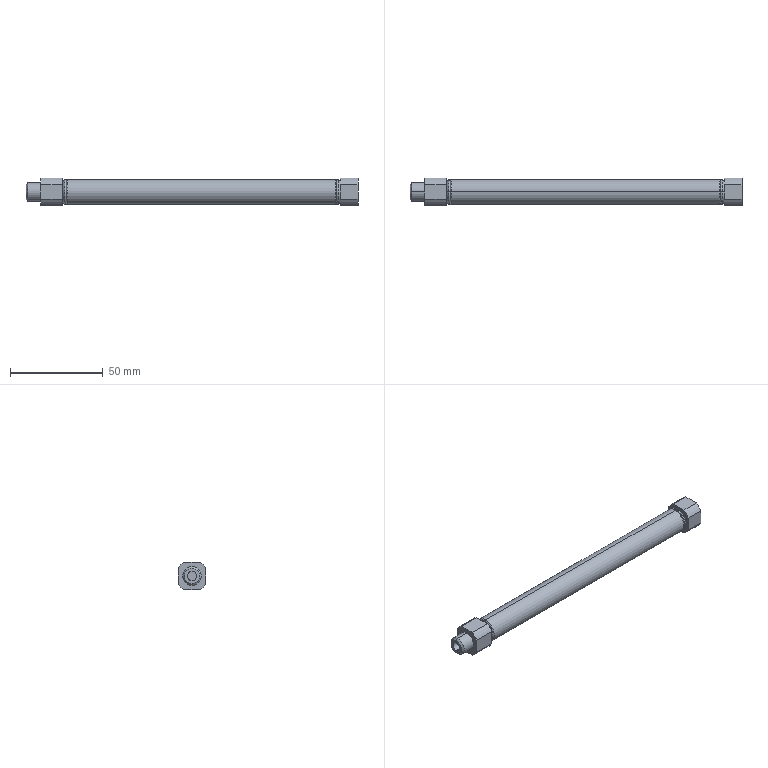Part | STEP file | 001-004-12PB125UBody | 1 solid | 64 faces | box 179 x 15 x 15 mm | volume 9809 mm3 | cylinder 24 | plane 18 | cone 14 | torus 8 | commonest cylinder face diameters 17 x8 4.134 x4 13.8 x4 5 x2 10 x2 12 x2